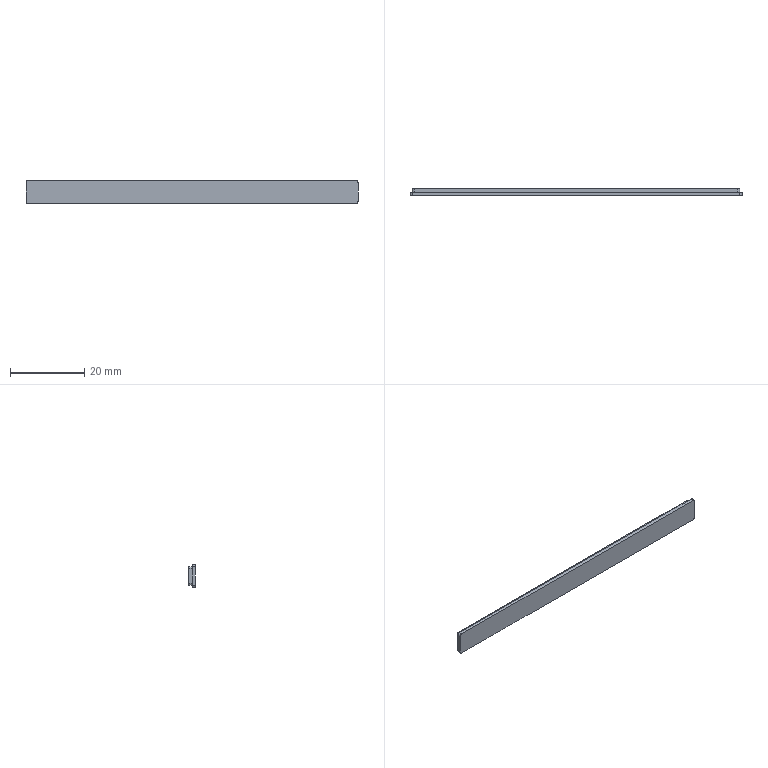Part | SolidWorks | features BaseBody 1 | 1 solid | 19 faces | box 89.3 x 1.85 x 6.3 mm | volume 917.679 mm3 | plane 11 | cylinder 8 | commonest cylinder face diameters 1 x4 1.3 x4
STEP:
#1=CARTESIAN_POINT('',(44.65,1.15,-2.5));
#2=VERTEX_POINT('',#1);
#3=CARTESIAN_POINT('',(44.65,1.15,2.5));
#4=VERTEX_POINT('',#3);
#5=CARTESIAN_POINT('',(44.65,1.15,-2.5));
#6=DIRECTION('',(0.,0.,1.));
#7=VECTOR('',#6,1000.);
#8=LINE('',#5,#7);
#9=EDGE_CURVE('',#2,#4,#8,.T.);
#10=ORIENTED_EDGE('',*,*,#9,.T.);
#11=CARTESIAN_POINT('',(44.,1.15,3.15));
#12=VERTEX_POINT('',#11);
#13=CARTESIAN_POINT('',(44.,1.15,2.5));
#14=DIRECTION('',(0.,-1.,0.));
#15=DIRECTION('',(0.,0.,1.));
#16=AXIS2_PLACEMENT_3D('',#13,#14,#15);
#17=CIRCLE('',#16,0.65);
#18=EDGE_CURVE('',#4,#12,#17,.T.);
#19=ORIENTED_EDGE('',*,*,#18,.T.);
#20=CARTESIAN_POINT('',(-44.,1.15,3.15));
#21=VERTEX_POINT('',#20);
#22=CARTESIAN_POINT('',(-44.,1.15,3.15));
#23=DIRECTION('',(-1.,0.,0.));
#24=VECTOR('',#23,1000.);
#25=LINE('',#22,#24);
#26=EDGE_CURVE('',#12,#21,#25,.T.);
#27=ORIENTED_EDGE('',*,*,#26,.T.);
#28=CARTESIAN_POINT('',(-44.65,1.15,2.5));
#29=VERTEX_POINT('',#28);
#30=CARTESIAN_POINT('',(-44.,1.15,2.5));
#31=DIRECTION('',(0.,-1.,0.));
#32=DIRECTION('',(0.,0.,1.));
#33=AXIS2_PLACEMENT_3D('',#30,#31,#32);
#34=CIRCLE('',#33,0.65);
#35=EDGE_CURVE('',#21,#29,#34,.T.);
#36=ORIENTED_EDGE('',*,*,#35,.T.);
#37=CARTESIAN_POINT('',(-44.65,1.15,-2.5));
#38=VERTEX_POINT('',#37);
#39=CARTESIAN_POINT('',(-44.65,1.15,-2.5));
#40=DIRECTION('',(0.,0.,-1.));
#41=VECTOR('',#40,1000.);
#42=LINE('',#39,#41);
#43=EDGE_CURVE('',#29,#38,#42,.T.);
#44=ORIENTED_EDGE('',*,*,#43,.T.);
#45=CARTESIAN_POINT('',(-44.,1.15,-3.15));
#46=VERTEX_POINT('',#45);
#47=CARTESIAN_POINT('',(-44.,1.15,-2.5));
#48=DIRECTION('',(0.,-1.,0.));
#49=DIRECTION('',(0.,0.,1.));
#50=AXIS2_PLACEMENT_3D('',#47,#48,#49);
#51=CIRCLE('',#50,0.65);
#52=EDGE_CURVE('',#38,#46,#51,.T.);
#53=ORIENTED_EDGE('',*,*,#52,.T.);
#54=CARTESIAN_POINT('',(44.,1.15,-3.15));
#55=VERTEX_POINT('',#54);
#56=CARTESIAN_POINT('',(-44.,1.15,-3.15));
#57=DIRECTION('',(1.,0.,0.));
#58=VECTOR('',#57,1000.);
#59=LINE('',#56,#58);
#60=EDGE_CURVE('',#46,#55,#59,.T.);
#61=ORIENTED_EDGE('',*,*,#60,.T.);
#62=CARTESIAN_POINT('',(44.,1.15,-2.5));
#63=DIRECTION('',(0.,-1.,0.));
#64=DIRECTION('',(0.,0.,1.));
#65=AXIS2_PLACEMENT_3D('',#62,#63,#64);
#66=CIRCLE('',#65,0.65);
#67=EDGE_CURVE('',#55,#2,#66,.T.);
#68=ORIENTED_EDGE('',*,*,#67,.T.);
#69=EDGE_LOOP('',(#10,#19,#27,#36,#44,#53,#61,#68));
#70=FACE_OUTER_BOUND('',#69,.T.);
#71=CARTESIAN_POINT('',(-44.,1.15,-2.5));
#72=DIRECTION('',(0.,-1.,0.));
#73=DIRECTION('',(0.,0.,-1.));
#74=AXIS2_PLACEMENT_3D('',#71,#72,#73);
#75=PLANE('',#74);
#76=ADVANCED_FACE('',(#70),#75,.T.);
#77=CARTESIAN_POINT('',(44.,2.,3.15));
#78=VERTEX_POINT('',#77);
#79=CARTESIAN_POINT('',(44.,0.,3.15));
#80=DIRECTION('',(0.,-1.,0.));
#81=VECTOR('',#80,1000.);
#82=LINE('',#79,#81);
#83=EDGE_CURVE('',#78,#12,#82,.T.);
#84=ORIENTED_EDGE('',*,*,#83,.T.);
#85=ORIENTED_EDGE('',*,*,#18,.F.);
#86=CARTESIAN_POINT('',(44.65,2.,2.5));
#87=VERTEX_POINT('',#86);
#88=CARTESIAN_POINT('',(44.65,0.,2.5));
#89=DIRECTION('',(0.,1.,0.));
#90=VECTOR('',#89,1000.);
#91=LINE('',#88,#90);
#92=EDGE_CURVE('',#4,#87,#91,.T.);
#93=ORIENTED_EDGE('',*,*,#92,.T.);
#94=CARTESIAN_POINT('',(44.,2.,2.5));
#95=DIRECTION('',(0.,1.,0.));
#96=DIRECTION('',(0.,0.,1.));
#97=AXIS2_PLACEMENT_3D('',#94,#95,#96);
#98=CIRCLE('',#97,0.65);
#99=EDGE_CURVE('',#78,#87,#98,.T.);
#100=ORIENTED_EDGE('',*,*,#99,.F.);
#101=EDGE_LOOP('',(#84,#85,#93,#100));
#102=FACE_OUTER_BOUND('',#101,.T.);
#103=CARTESIAN_POINT('',(44.,0.,2.5));
#104=DIRECTION('',(0.,1.,0.));
#105=DIRECTION('',(0.,0.,1.));
#106=AXIS2_PLACEMENT_3D('',#103,#104,#105);
#107=CYLINDRICAL_SURFACE('',#106,0.65);
#108=ADVANCED_FACE('',(#102),#107,.T.);
#109=ORIENTED_EDGE('',*,*,#92,.F.);
#110=ORIENTED_EDGE('',*,*,#9,.F.);
#111=CARTESIAN_POINT('',(44.65,2.,-2.5));
#112=VERTEX_POINT('',#111);
#113=CARTESIAN_POINT('',(44.65,0.,-2.5));
#114=DIRECTION('',(0.,1.,0.));
#115=VECTOR('',#114,1000.);
#116=LINE('',#113,#115);
#117=EDGE_CURVE('',#2,#112,#116,.T.);
#118=ORIENTED_EDGE('',*,*,#117,.T.);
#119=CARTESIAN_POINT('',(44.65,2.,2.5));
#120=DIRECTION('',(0.,0.,1.));
#121=VECTOR('',#120,1000.);
#122=LINE('',#119,#121);
#123=EDGE_CURVE('',#112,#87,#122,.T.);
#124=ORIENTED_EDGE('',*,*,#123,.T.);
#125=EDGE_LOOP('',(#109,#110,#118,#124));
#126=FACE_OUTER_BOUND('',#125,.T.);
#127=CARTESIAN_POINT('',(44.65,0.,2.5));
#128=DIRECTION('',(1.,0.,0.));
#129=DIRECTION('',(0.,0.,-1.));
#130=AXIS2_PLACEMENT_3D('',#127,#128,#129);
#131=PLANE('',#130);
#132=ADVANCED_FACE('',(#126),#131,.T.);
#133=ORIENTED_EDGE('',*,*,#117,.F.);
#134=ORIENTED_EDGE('',*,*,#67,.F.);
#135=CARTESIAN_POINT('',(44.,2.,-3.15));
#136=VERTEX_POINT('',#135);
#137=CARTESIAN_POINT('',(44.,0.,-3.15));
#138=DIRECTION('',(0.,1.,0.));
#139=VECTOR('',#138,1000.);
#140=LINE('',#137,#139);
#141=EDGE_CURVE('',#55,#136,#140,.T.);
#142=ORIENTED_EDGE('',*,*,#141,.T.);
#143=CARTESIAN_POINT('',(44.,2.,-2.5));
#144=DIRECTION('',(0.,-1.,0.));
#145=DIRECTION('',(0.,0.,1.));
#146=AXIS2_PLACEMENT_3D('',#143,#144,#145);
#147=CIRCLE('',#146,0.65);
#148=EDGE_CURVE('',#136,#112,#147,.T.);
#149=ORIENTED_EDGE('',*,*,#148,.T.);
#150=EDGE_LOOP('',(#133,#134,#142,#149));
#151=FACE_OUTER_BOUND('',#150,.T.);
#152=CARTESIAN_POINT('',(44.,0.,-2.5));
#153=DIRECTION('',(0.,1.,0.));
#154=DIRECTION('',(0.,0.,1.));
#155=AXIS2_PLACEMENT_3D('',#152,#153,#154);
#156=CYLINDRICAL_SURFACE('',#155,0.65);
#157=ADVANCED_FACE('',(#151),#156,.T.);
#158=ORIENTED_EDGE('',*,*,#141,.F.);
#159=ORIENTED_EDGE('',*,*,#60,.F.);
#160=CARTESIAN_POINT('',(-44.,2.,-3.15));
#161=VERTEX_POINT('',#160);
#162=CARTESIAN_POINT('',(-44.,0.,-3.15));
#163=DIRECTION('',(0.,1.,0.));
#164=VECTOR('',#163,1000.);
#165=LINE('',#162,#164);
#166=EDGE_CURVE('',#46,#161,#165,.T.);
#167=ORIENTED_EDGE('',*,*,#166,.T.);
#168=CARTESIAN_POINT('',(44.,2.,-3.15));
#169=DIRECTION('',(1.,0.,0.));
#170=VECTOR('',#169,1000.);
#171=LINE('',#168,#170);
#172=EDGE_CURVE('',#161,#136,#171,.T.);
#173=ORIENTED_EDGE('',*,*,#172,.T.);
#174=EDGE_LOOP('',(#158,#159,#167,#173));
#175=FACE_OUTER_BOUND('',#174,.T.);
#176=CARTESIAN_POINT('',(44.,0.,-3.15));
#177=DIRECTION('',(0.,0.,-1.));
#178=DIRECTION('',(-1.,0.,0.));
#179=AXIS2_PLACEMENT_3D('',#176,#177,#178);
#180=PLANE('',#179);
#181=ADVANCED_FACE('',(#175),#180,.T.);
#182=ORIENTED_EDGE('',*,*,#166,.F.);
#183=ORIENTED_EDGE('',*,*,#52,.F.);
#184=CARTESIAN_POINT('',(-44.65,2.,-2.5));
#185=VERTEX_POINT('',#184);
#186=CARTESIAN_POINT('',(-44.65,0.,-2.5));
#187=DIRECTION('',(0.,1.,0.));
#188=VECTOR('',#187,1000.);
#189=LINE('',#186,#188);
#190=EDGE_CURVE('',#38,#185,#189,.T.);
#191=ORIENTED_EDGE('',*,*,#190,.T.);
#192=CARTESIAN_POINT('',(-44.,2.,-2.5));
#193=DIRECTION('',(0.,-1.,0.));
#194=DIRECTION('',(0.,0.,1.));
#195=AXIS2_PLACEMENT_3D('',#192,#193,#194);
#196=CIRCLE('',#195,0.65);
#197=EDGE_CURVE('',#185,#161,#196,.T.);
#198=ORIENTED_EDGE('',*,*,#197,.T.);
#199=EDGE_LOOP('',(#182,#183,#191,#198));
#200=FACE_OUTER_BOUND('',#199,.T.);
#201=CARTESIAN_POINT('',(-44.,0.,-2.5));
#202=DIRECTION('',(0.,1.,0.));
#203=DIRECTION('',(0.,0.,1.));
#204=AXIS2_PLACEMENT_3D('',#201,#202,#203);
#205=CYLINDRICAL_SURFACE('',#204,0.65);
#206=ADVANCED_FACE('',(#200),#205,.T.);
#207=ORIENTED_EDGE('',*,*,#190,.F.);
#208=ORIENTED_EDGE('',*,*,#43,.F.);
#209=CARTESIAN_POINT('',(-44.65,2.,2.5));
#210=VERTEX_POINT('',#209);
#211=CARTESIAN_POINT('',(-44.65,0.,2.5));
#212=DIRECTION('',(0.,1.,0.));
#213=VECTOR('',#212,1000.);
#214=LINE('',#211,#213);
#215=EDGE_CURVE('',#29,#210,#214,.T.);
#216=ORIENTED_EDGE('',*,*,#215,.T.);
#217=CARTESIAN_POINT('',(-44.65,2.,-2.5));
#218=DIRECTION('',(0.,0.,-1.));
#219=VECTOR('',#218,1000.);
#220=LINE('',#217,#219);
#221=EDGE_CURVE('',#210,#185,#220,.T.);
#222=ORIENTED_EDGE('',*,*,#221,.T.);
#223=EDGE_LOOP('',(#207,#208,#216,#222));
#224=FACE_OUTER_BOUND('',#223,.T.);
#225=CARTESIAN_POINT('',(-44.65,0.,-2.5));
#226=DIRECTION('',(-1.,0.,0.));
#227=DIRECTION('',(0.,0.,1.));
#228=AXIS2_PLACEMENT_3D('',#225,#226,#227);
#229=PLANE('',#228);
#230=ADVANCED_FACE('',(#224),#229,.T.);
#231=ORIENTED_EDGE('',*,*,#215,.F.);
#232=ORIENTED_EDGE('',*,*,#35,.F.);
#233=CARTESIAN_POINT('',(-44.,2.,3.15));
#234=VERTEX_POINT('',#233);
#235=CARTESIAN_POINT('',(-44.,0.,3.15));
#236=DIRECTION('',(0.,1.,0.));
#237=VECTOR('',#236,1000.);
#238=LINE('',#235,#237);
#239=EDGE_CURVE('',#21,#234,#238,.T.);
#240=ORIENTED_EDGE('',*,*,#239,.T.);
#241=CARTESIAN_POINT('',(-44.,2.,2.5));
#242=DIRECTION('',(0.,-1.,0.));
#243=DIRECTION('',(0.,0.,1.));
#244=AXIS2_PLACEMENT_3D('',#241,#242,#243);
#245=CIRCLE('',#244,0.65);
#246=EDGE_CURVE('',#234,#210,#245,.T.);
#247=ORIENTED_EDGE('',*,*,#246,.T.);
#248=EDGE_LOOP('',(#231,#232,#240,#247));
#249=FACE_OUTER_BOUND('',#248,.T.);
#250=CARTESIAN_POINT('',(-44.,0.,2.5));
#251=DIRECTION('',(0.,1.,0.));
#252=DIRECTION('',(0.,0.,1.));
#253=AXIS2_PLACEMENT_3D('',#250,#251,#252);
#254=CYLINDRICAL_SURFACE('',#253,0.65);
#255=ADVANCED_FACE('',(#249),#254,.T.);
#256=ORIENTED_EDGE('',*,*,#239,.F.);
#257=ORIENTED_EDGE('',*,*,#26,.F.);
#258=ORIENTED_EDGE('',*,*,#83,.F.);
#259=CARTESIAN_POINT('',(-44.,2.,3.15));
#260=DIRECTION('',(-1.,0.,0.));
#261=VECTOR('',#260,1000.);
#262=LINE('',#259,#261);
#263=EDGE_CURVE('',#78,#234,#262,.T.);
#264=ORIENTED_EDGE('',*,*,#263,.T.);
#265=EDGE_LOOP('',(#256,#257,#258,#264));
#266=FACE_OUTER_BOUND('',#265,.T.);
#267=CARTESIAN_POINT('',(-44.,0.,3.15));
#268=DIRECTION('',(0.,0.,1.));
#269=DIRECTION('',(1.,0.,0.));
#270=AXIS2_PLACEMENT_3D('',#267,#268,#269);
#271=PLANE('',#270);
#272=ADVANCED_FACE('',(#266),#271,.T.);
#273=ORIENTED_EDGE('',*,*,#172,.F.);
#274=ORIENTED_EDGE('',*,*,#197,.F.);
#275=ORIENTED_EDGE('',*,*,#221,.F.);
#276=ORIENTED_EDGE('',*,*,#246,.F.);
#277=ORIENTED_EDGE('',*,*,#263,.F.);
#278=ORIENTED_EDGE('',*,*,#99,.T.);
#279=ORIENTED_EDGE('',*,*,#123,.F.);
#280=ORIENTED_EDGE('',*,*,#148,.F.);
#281=EDGE_LOOP('',(#273,#274,#275,#276,#277,#278,#279,#280));
#282=FACE_OUTER_BOUND('',#281,.T.);
#283=CARTESIAN_POINT('',(43.5,2.,2.5));
#284=VERTEX_POINT('',#283);
#285=CARTESIAN_POINT('',(-43.5,2.,2.5));
#286=VERTEX_POINT('',#285);
#287=CARTESIAN_POINT('',(0.,2.,2.5));
#288=DIRECTION('',(-1.,0.,0.));
#289=VECTOR('',#288,1000.);
#290=LINE('',#287,#289);
#291=EDGE_CURVE('',#284,#286,#290,.T.);
#292=ORIENTED_EDGE('',*,*,#291,.T.);
#293=CARTESIAN_POINT('',(-44.,2.,2.));
#294=VERTEX_POINT('',#293);
#295=CARTESIAN_POINT('',(-43.5,2.,2.));
#296=DIRECTION('',(0.,-1.,0.));
#297=DIRECTION('',(0.,0.,-1.));
#298=AXIS2_PLACEMENT_3D('',#295,#296,#297);
#299=CIRCLE('',#298,0.5);
#300=EDGE_CURVE('',#286,#294,#299,.T.);
#301=ORIENTED_EDGE('',*,*,#300,.T.);
#302=CARTESIAN_POINT('',(-44.,2.,-2.));
#303=VERTEX_POINT('',#302);
#304=CARTESIAN_POINT('',(-44.,2.,0.));
#305=DIRECTION('',(0.,0.,-1.));
#306=VECTOR('',#305,1000.);
#307=LINE('',#304,#306);
#308=EDGE_CURVE('',#294,#303,#307,.T.);
#309=ORIENTED_EDGE('',*,*,#308,.T.);
#310=CARTESIAN_POINT('',(-43.5,2.,-2.5));
#311=VERTEX_POINT('',#310);
#312=CARTESIAN_POINT('',(-43.5,2.,-2.));
#313=DIRECTION('',(0.,-1.,0.));
#314=DIRECTION('',(0.,0.,-1.));
#315=AXIS2_PLACEMENT_3D('',#312,#313,#314);
#316=CIRCLE('',#315,0.5);
#317=EDGE_CURVE('',#303,#311,#316,.T.);
#318=ORIENTED_EDGE('',*,*,#317,.T.);
#319=CARTESIAN_POINT('',(43.5,2.,-2.5));
#320=VERTEX_POINT('',#319);
#321=CARTESIAN_POINT('',(0.,2.,-2.5));
#322=DIRECTION('',(1.,0.,0.));
#323=VECTOR('',#322,1000.);
#324=LINE('',#321,#323);
#325=EDGE_CURVE('',#311,#320,#324,.T.);
#326=ORIENTED_EDGE('',*,*,#325,.T.);
#327=CARTESIAN_POINT('',(44.,2.,-2.));
#328=VERTEX_POINT('',#327);
#329=CARTESIAN_POINT('',(43.5,2.,-2.));
#330=DIRECTION('',(0.,-1.,0.));
#331=DIRECTION('',(0.,0.,-1.));
#332=AXIS2_PLACEMENT_3D('',#329,#330,#331);
#333=CIRCLE('',#332,0.5);
#334=EDGE_CURVE('',#320,#328,#333,.T.);
#335=ORIENTED_EDGE('',*,*,#334,.T.);
#336=CARTESIAN_POINT('',(44.,2.,2.));
#337=VERTEX_POINT('',#336);
#338=CARTESIAN_POINT('',(44.,2.,0.));
#339=DIRECTION('',(0.,0.,1.));
#340=VECTOR('',#339,1000.);
#341=LINE('',#338,#340);
#342=EDGE_CURVE('',#328,#337,#341,.T.);
#343=ORIENTED_EDGE('',*,*,#342,.T.);
#344=CARTESIAN_POINT('',(43.5,2.,2.));
#345=DIRECTION('',(0.,-1.,0.));
#346=DIRECTION('',(0.,0.,-1.));
#347=AXIS2_PLACEMENT_3D('',#344,#345,#346);
#348=CIRCLE('',#347,0.5);
#349=EDGE_CURVE('',#337,#284,#348,.T.);
#350=ORIENTED_EDGE('',*,*,#349,.T.);
#351=EDGE_LOOP('',(#292,#301,#309,#318,#326,#335,#343,#350));
#352=FACE_BOUND('',#351,.T.);
#353=CARTESIAN_POINT('',(0.,2.,0.));
#354=DIRECTION('',(0.,1.,0.));
#355=DIRECTION('',(0.,0.,1.));
#356=AXIS2_PLACEMENT_3D('',#353,#354,#355);
#357=PLANE('',#356);
#358=ADVANCED_FACE('',(#282,#352),#357,.T.);
#359=ORIENTED_EDGE('',*,*,#300,.F.);
#360=CARTESIAN_POINT('',(-43.5,3.,2.5));
#361=VERTEX_POINT('',#360);
#362=CARTESIAN_POINT('',(-43.5,3.,2.5));
#363=DIRECTION('',(0.,1.,0.));
#364=VECTOR('',#363,1000.);
#365=LINE('',#362,#364);
#366=EDGE_CURVE('',#286,#361,#365,.T.);
#367=ORIENTED_EDGE('',*,*,#366,.T.);
#368=CARTESIAN_POINT('',(-44.,3.,2.));
#369=VERTEX_POINT('',#368);
#370=CARTESIAN_POINT('',(-43.5,3.,2.));
#371=DIRECTION('',(0.,1.,0.));
#372=DIRECTION('',(0.,0.,-1.));
#373=AXIS2_PLACEMENT_3D('',#370,#371,#372);
#374=CIRCLE('',#373,0.5);
#375=EDGE_CURVE('',#369,#361,#374,.T.);
#376=ORIENTED_EDGE('',*,*,#375,.F.);
#377=CARTESIAN_POINT('',(-44.,3.,2.));
#378=DIRECTION('',(0.,-1.,0.));
#379=VECTOR('',#378,1000.);
#380=LINE('',#377,#379);
#381=EDGE_CURVE('',#369,#294,#380,.T.);
#382=ORIENTED_EDGE('',*,*,#381,.T.);
#383=EDGE_LOOP('',(#359,#367,#376,#382));
#384=FACE_OUTER_BOUND('',#383,.T.);
#385=CARTESIAN_POINT('',(-43.5,3.,2.));
#386=DIRECTION('',(0.,-1.,0.));
#387=DIRECTION('',(0.,0.,-1.));
#388=AXIS2_PLACEMENT_3D('',#385,#386,#387);
#389=CYLINDRICAL_SURFACE('',#388,0.5);
#390=ADVANCED_FACE('',(#384),#389,.T.);
#391=CARTESIAN_POINT('',(43.5,3.,2.5));
#392=VERTEX_POINT('',#391);
#393=CARTESIAN_POINT('',(43.5,3.,2.5));
#394=DIRECTION('',(0.,-1.,0.));
#395=VECTOR('',#394,1000.);
#396=LINE('',#393,#395);
#397=EDGE_CURVE('',#392,#284,#396,.T.);
#398=ORIENTED_EDGE('',*,*,#397,.F.);
#399=CARTESIAN_POINT('',(44.,3.,2.5));
#400=DIRECTION('',(1.,0.,0.));
#401=VECTOR('',#400,1000.);
#402=LINE('',#399,#401);
#403=EDGE_CURVE('',#361,#392,#402,.T.);
#404=ORIENTED_EDGE('',*,*,#403,.F.);
#405=ORIENTED_EDGE('',*,*,#366,.F.);
#406=ORIENTED_EDGE('',*,*,#291,.F.);
#407=EDGE_LOOP('',(#398,#404,#405,#406));
#408=FACE_OUTER_BOUND('',#407,.T.);
#409=CARTESIAN_POINT('',(44.,3.,2.5));
#410=DIRECTION('',(0.,0.,-1.));
#411=DIRECTION('',(-1.,0.,0.));
#412=AXIS2_PLACEMENT_3D('',#409,#410,#411);
#413=PLANE('',#412);
#414=ADVANCED_FACE('',(#408),#413,.F.);
#415=ORIENTED_EDGE('',*,*,#349,.F.);
#416=CARTESIAN_POINT('',(44.,3.,2.));
#417=VERTEX_POINT('',#416);
#418=CARTESIAN_POINT('',(44.,3.,2.));
#419=DIRECTION('',(0.,1.,0.));
#420=VECTOR('',#419,1000.);
#421=LINE('',#418,#420);
#422=EDGE_CURVE('',#337,#417,#421,.T.);
#423=ORIENTED_EDGE('',*,*,#422,.T.);
#424=CARTESIAN_POINT('',(43.5,3.,2.));
#425=DIRECTION('',(0.,-1.,0.));
#426=DIRECTION('',(0.,0.,-1.));
#427=AXIS2_PLACEMENT_3D('',#424,#425,#426);
#428=CIRCLE('',#427,0.5);
#429=EDGE_CURVE('',#417,#392,#428,.T.);
#430=ORIENTED_EDGE('',*,*,#429,.T.);
#431=ORIENTED_EDGE('',*,*,#397,.T.);
#432=EDGE_LOOP('',(#415,#423,#430,#431));
#433=FACE_OUTER_BOUND('',#432,.T.);
#434=CARTESIAN_POINT('',(43.5,3.,2.));
#435=DIRECTION('',(0.,-1.,0.));
#436=DIRECTION('',(0.,0.,-1.));
#437=AXIS2_PLACEMENT_3D('',#434,#435,#436);
#438=CYLINDRICAL_SURFACE('',#437,0.5);
#439=ADVANCED_FACE('',(#433),#438,.T.);
#440=ORIENTED_EDGE('',*,*,#422,.F.);
#441=ORIENTED_EDGE('',*,*,#342,.F.);
#442=CARTESIAN_POINT('',(44.,3.,-2.));
#443=VERTEX_POINT('',#442);
#444=CARTESIAN_POINT('',(44.,3.,-2.));
#445=DIRECTION('',(0.,-1.,0.));
#446=VECTOR('',#445,1000.);
#447=LINE('',#444,#446);
#448=EDGE_CURVE('',#443,#328,#447,.T.);
#449=ORIENTED_EDGE('',*,*,#448,.F.);
#450=CARTESIAN_POINT('',(44.,3.,2.5));
#451=DIRECTION('',(0.,0.,-1.));
#452=VECTOR('',#451,1000.);
#453=LINE('',#450,#452);
#454=EDGE_CURVE('',#417,#443,#453,.T.);
#455=ORIENTED_EDGE('',*,*,#454,.F.);
#456=EDGE_LOOP('',(#440,#441,#449,#455));
#457=FACE_OUTER_BOUND('',#456,.T.);
#458=CARTESIAN_POINT('',(44.,3.,2.5));
#459=DIRECTION('',(-1.,0.,0.));
#460=DIRECTION('',(0.,0.,1.));
#461=AXIS2_PLACEMENT_3D('',#458,#459,#460);
#462=PLANE('',#461);
#463=ADVANCED_FACE('',(#457),#462,.F.);
#464=ORIENTED_EDGE('',*,*,#334,.F.);
#465=CARTESIAN_POINT('',(43.5,3.,-2.5));
#466=VERTEX_POINT('',#465);
#467=CARTESIAN_POINT('',(43.5,3.,-2.5));
#468=DIRECTION('',(0.,1.,0.));
#469=VECTOR('',#468,1000.);
#470=LINE('',#467,#469);
#471=EDGE_CURVE('',#320,#466,#470,.T.);
#472=ORIENTED_EDGE('',*,*,#471,.T.);
#473=CARTESIAN_POINT('',(43.5,3.,-2.));
#474=DIRECTION('',(0.,-1.,0.));
#475=DIRECTION('',(0.,0.,-1.));
#476=AXIS2_PLACEMENT_3D('',#473,#474,#475);
#477=CIRCLE('',#476,0.5);
#478=EDGE_CURVE('',#466,#443,#477,.T.);
#479=ORIENTED_EDGE('',*,*,#478,.T.);
#480=ORIENTED_EDGE('',*,*,#448,.T.);
#481=EDGE_LOOP('',(#464,#472,#479,#480));
#482=FACE_OUTER_BOUND('',#481,.T.);
#483=CARTESIAN_POINT('',(43.5,3.,-2.));
#484=DIRECTION('',(0.,-1.,0.));
#485=DIRECTION('',(0.,0.,-1.));
#486=AXIS2_PLACEMENT_3D('',#483,#484,#485);
#487=CYLINDRICAL_SURFACE('',#486,0.5);
#488=ADVANCED_FACE('',(#482),#487,.T.);
#489=ORIENTED_EDGE('',*,*,#471,.F.);
#490=ORIENTED_EDGE('',*,*,#325,.F.);
#491=CARTESIAN_POINT('',(-43.5,3.,-2.5));
#492=VERTEX_POINT('',#491);
#493=CARTESIAN_POINT('',(-43.5,3.,-2.5));
#494=DIRECTION('',(0.,-1.,0.));
#495=VECTOR('',#494,1000.);
#496=LINE('',#493,#495);
#497=EDGE_CURVE('',#492,#311,#496,.T.);
#498=ORIENTED_EDGE('',*,*,#497,.F.);
#499=CARTESIAN_POINT('',(44.,3.,-2.5));
#500=DIRECTION('',(-1.,0.,0.));
#501=VECTOR('',#500,1000.);
#502=LINE('',#499,#501);
#503=EDGE_CURVE('',#466,#492,#502,.T.);
#504=ORIENTED_EDGE('',*,*,#503,.F.);
#505=EDGE_LOOP('',(#489,#490,#498,#504));
#506=FACE_OUTER_BOUND('',#505,.T.);
#507=CARTESIAN_POINT('',(44.,3.,-2.5));
#508=DIRECTION('',(0.,0.,1.));
#509=DIRECTION('',(1.,0.,0.));
#510=AXIS2_PLACEMENT_3D('',#507,#508,#509);
#511=PLANE('',#510);
#512=ADVANCED_FACE('',(#506),#511,.F.);
#513=ORIENTED_EDGE('',*,*,#317,.F.);
#514=CARTESIAN_POINT('',(-44.,3.,-2.));
#515=VERTEX_POINT('',#514);
#516=CARTESIAN_POINT('',(-44.,3.,-2.));
#517=DIRECTION('',(0.,1.,0.));
#518=VECTOR('',#517,1000.);
#519=LINE('',#516,#518);
#520=EDGE_CURVE('',#303,#515,#519,.T.);
#521=ORIENTED_EDGE('',*,*,#520,.T.);
#522=CARTESIAN_POINT('',(-43.5,3.,-2.));
#523=DIRECTION('',(0.,-1.,0.));
#524=DIRECTION('',(0.,0.,-1.));
#525=AXIS2_PLACEMENT_3D('',#522,#523,#524);
#526=CIRCLE('',#525,0.5);
#527=EDGE_CURVE('',#515,#492,#526,.T.);
#528=ORIENTED_EDGE('',*,*,#527,.T.);
#529=ORIENTED_EDGE('',*,*,#497,.T.);
#530=EDGE_LOOP('',(#513,#521,#528,#529));
#531=FACE_OUTER_BOUND('',#530,.T.);
#532=CARTESIAN_POINT('',(-43.5,3.,-2.));
#533=DIRECTION('',(0.,-1.,0.));
#534=DIRECTION('',(0.,0.,-1.));
#535=AXIS2_PLACEMENT_3D('',#532,#533,#534);
#536=CYLINDRICAL_SURFACE('',#535,0.5);
#537=ADVANCED_FACE('',(#531),#536,.T.);
#538=ORIENTED_EDGE('',*,*,#520,.F.);
#539=ORIENTED_EDGE('',*,*,#308,.F.);
#540=ORIENTED_EDGE('',*,*,#381,.F.);
#541=CARTESIAN_POINT('',(-44.,3.,2.5));
#542=DIRECTION('',(0.,0.,1.));
#543=VECTOR('',#542,1000.);
#544=LINE('',#541,#543);
#545=EDGE_CURVE('',#515,#369,#544,.T.);
#546=ORIENTED_EDGE('',*,*,#545,.F.);
#547=EDGE_LOOP('',(#538,#539,#540,#546));
#548=FACE_OUTER_BOUND('',#547,.T.);
#549=CARTESIAN_POINT('',(-44.,3.,2.5));
#550=DIRECTION('',(1.,0.,0.));
#551=DIRECTION('',(0.,0.,-1.));
#552=AXIS2_PLACEMENT_3D('',#549,#550,#551);
#553=PLANE('',#552);
#554=ADVANCED_FACE('',(#548),#553,.F.);
#555=ORIENTED_EDGE('',*,*,#545,.T.);
#556=ORIENTED_EDGE('',*,*,#375,.T.);
#557=ORIENTED_EDGE('',*,*,#403,.T.);
#558=ORIENTED_EDGE('',*,*,#429,.F.);
#559=ORIENTED_EDGE('',*,*,#454,.T.);
#560=ORIENTED_EDGE('',*,*,#478,.F.);
#561=ORIENTED_EDGE('',*,*,#503,.T.);
#562=ORIENTED_EDGE('',*,*,#527,.F.);
#563=EDGE_LOOP('',(#555,#556,#557,#558,#559,#560,#561,#562));
#564=FACE_OUTER_BOUND('',#563,.T.);
#565=CARTESIAN_POINT('',(0.,3.,0.));
#566=DIRECTION('',(0.,1.,0.));
#567=DIRECTION('',(0.,0.,1.));
#568=AXIS2_PLACEMENT_3D('',#565,#566,#567);
#569=PLANE('',#568);
#570=ADVANCED_FACE('',(#564),#569,.T.);
#571=CLOSED_SHELL('',(#76,#108,#132,#157,#181,#206,#230,#255,#272,#358,#390,#414,#439,#463,#488,#512,#537,#554,#570));
#572=MANIFOLD_SOLID_BREP('',#571);
#573=CARTESIAN_POINT('',(0.,0.,0.));
#574=DIRECTION('',(0.,0.,1.));
#575=DIRECTION('',(1.,0.,0.));
#576=AXIS2_PLACEMENT_3D('',#573,#574,#575);
#577=(LENGTH_UNIT()NAMED_UNIT(*)SI_UNIT(.MILLI.,.METRE.));
#578=UNCERTAINTY_MEASURE_WITH_UNIT(LENGTH_MEASURE(0.00001),#577,'','');
#579=(NAMED_UNIT(*)PLANE_ANGLE_UNIT()SI_UNIT($,.RADIAN.));
#580=(NAMED_UNIT(*)SI_UNIT($,.STERADIAN.)SOLID_ANGLE_UNIT());
#581=(GEOMETRIC_REPRESENTATION_CONTEXT(3)GLOBAL_UNCERTAINTY_ASSIGNED_CONTEXT((#578))GLOBAL_UNIT_ASSIGNED_CONTEXT((#577,#579,#580))REPRESENTATION_CONTEXT('',''));
#582=ADVANCED_BREP_SHAPE_REPRESENTATION('',(#572,#576),#581);